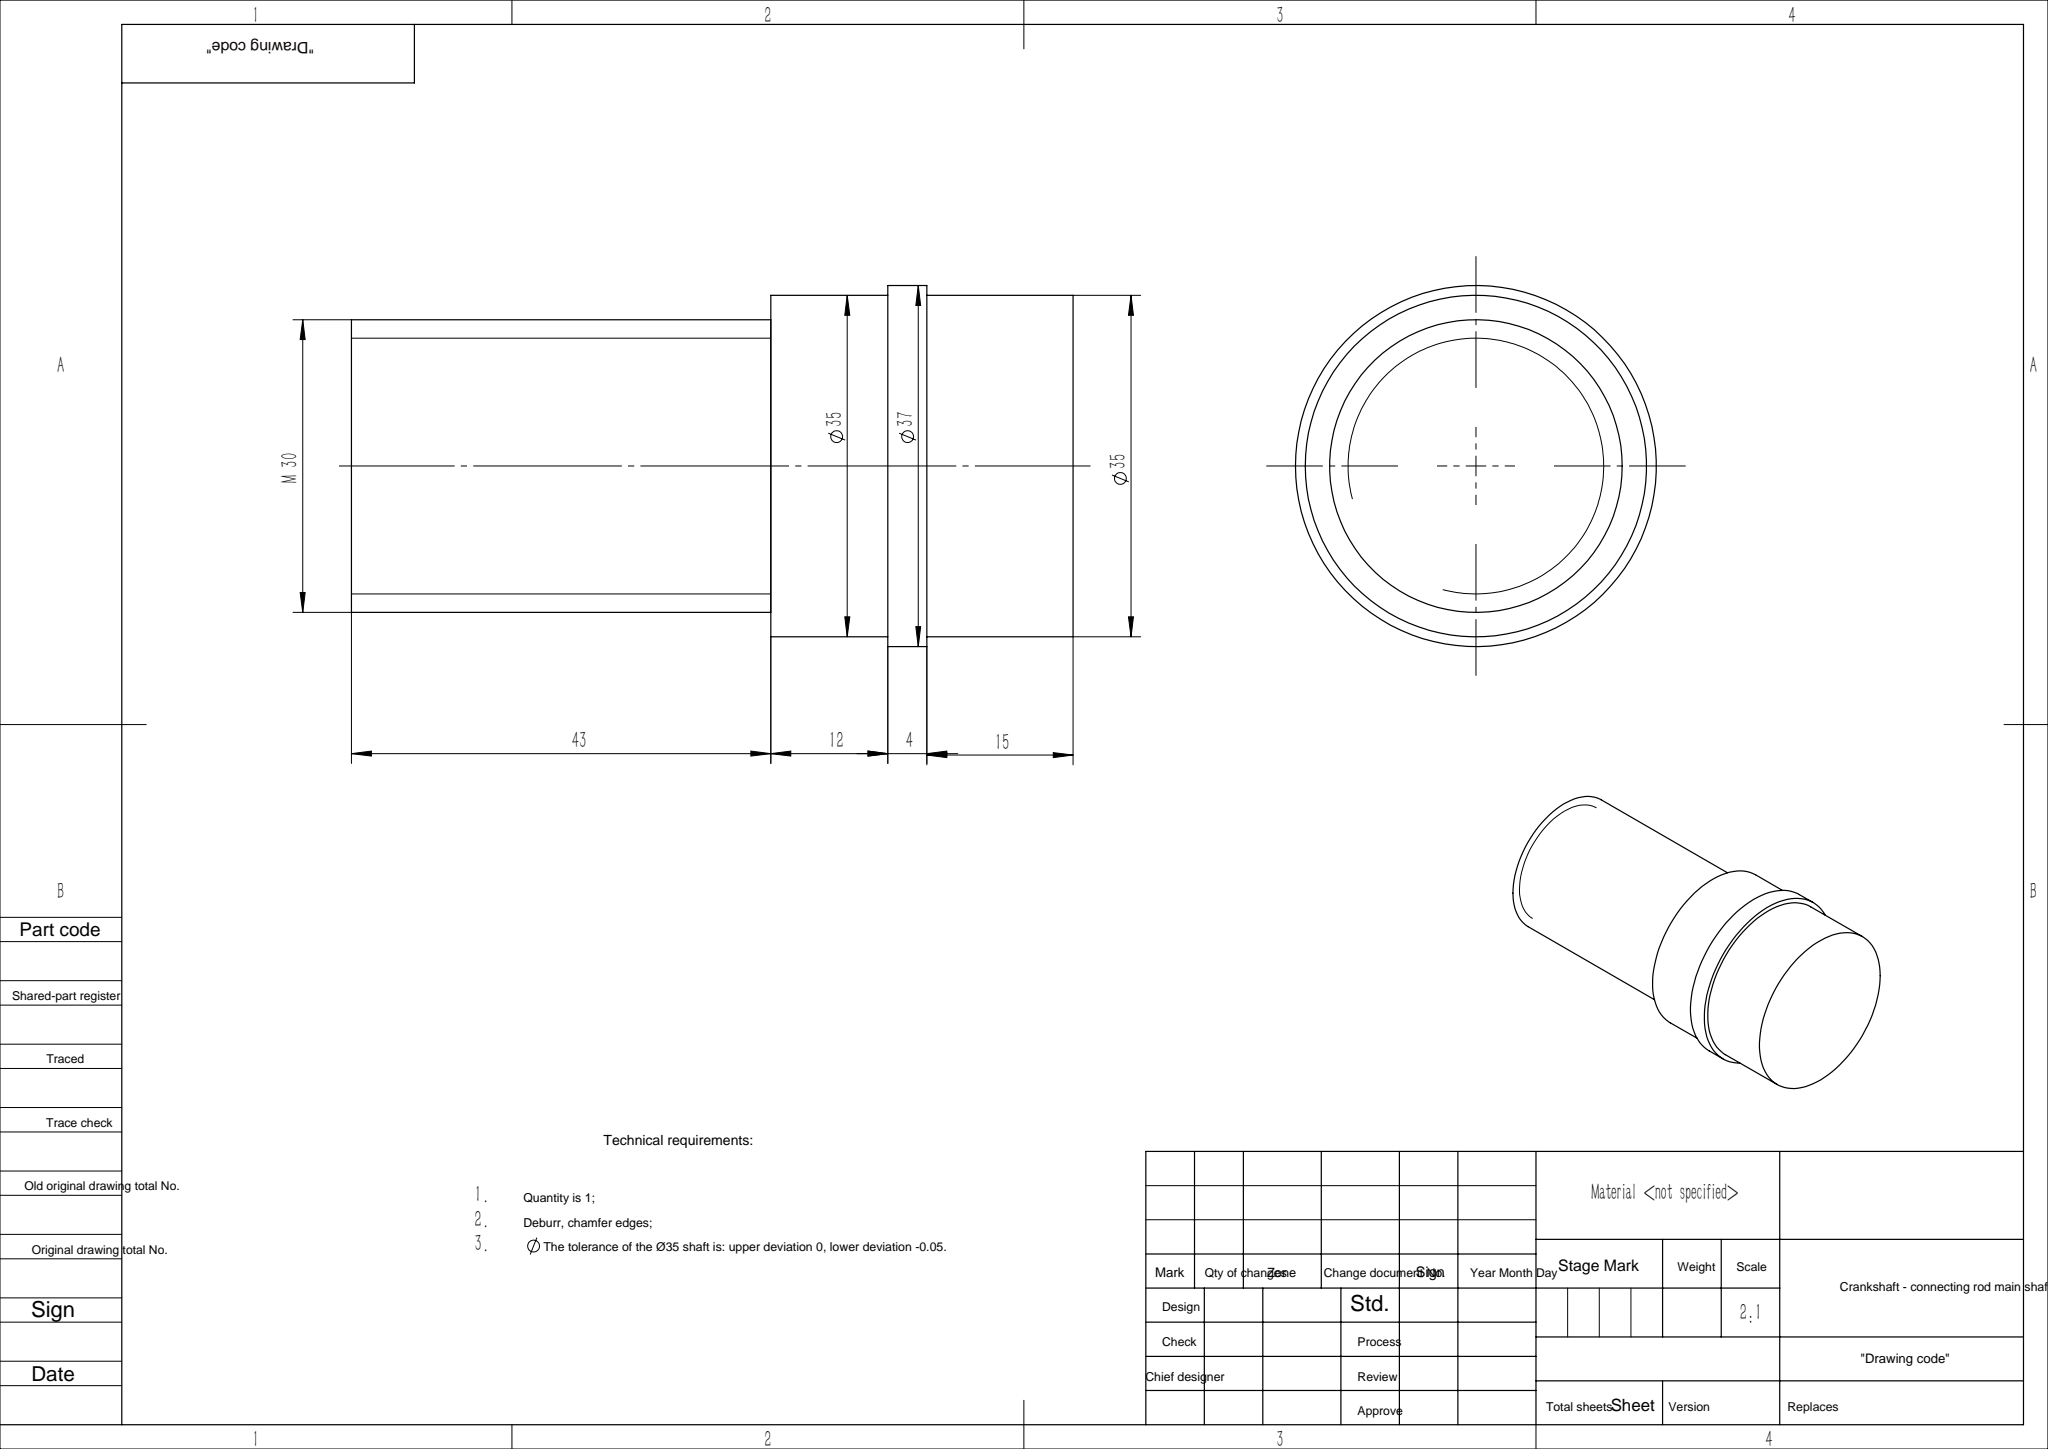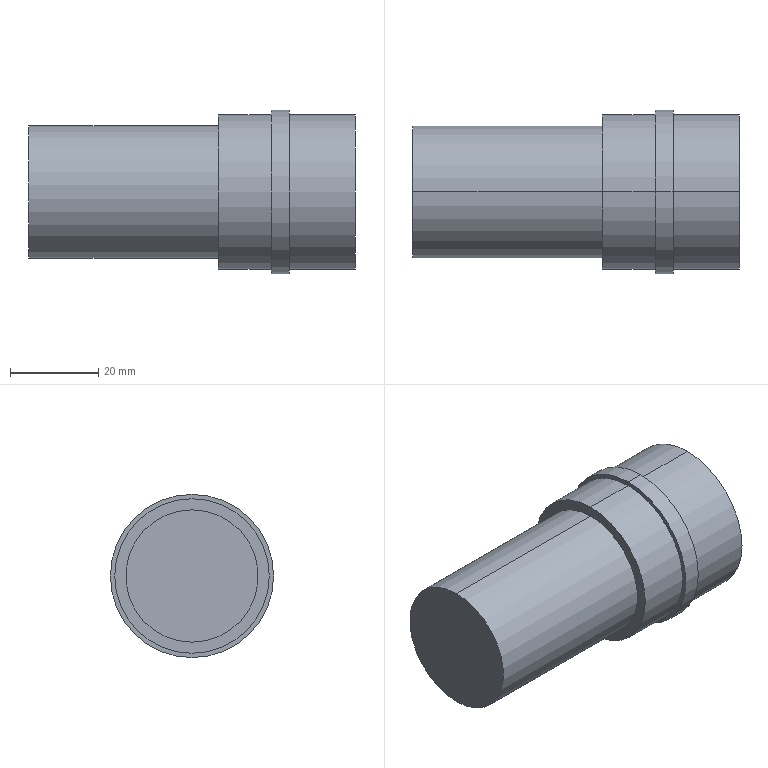Part | SolidWorks | features ICE 2, Extrusion 1 | 1 solid | 13 faces | box 74 x 37 x 37 mm | volume 60673 mm3 | cylinder 8 | plane 5 | commonest cylinder face diameters 35 x4 30 x2 37 x2
STEP:
#1=CARTESIAN_POINT('',(31.,0.,-17.5));
#2=VERTEX_POINT('',#1);
#3=CARTESIAN_POINT('',(31.,0.,17.5));
#4=VERTEX_POINT('',#3);
#5=CARTESIAN_POINT('',(31.,0.,0.));
#6=DIRECTION('',(1.,0.,0.));
#7=DIRECTION('',(0.,0.,-1.));
#8=AXIS2_PLACEMENT_3D('',#5,#6,#7);
#9=CIRCLE('',#8,17.5);
#10=EDGE_CURVE('',#2,#4,#9,.T.);
#11=ORIENTED_EDGE('',*,*,#10,.F.);
#12=CARTESIAN_POINT('',(16.,0.,-17.5));
#13=VERTEX_POINT('',#12);
#14=CARTESIAN_POINT('',(31.,0.,-17.5));
#15=DIRECTION('',(-1.,0.,0.));
#16=VECTOR('',#15,1000.);
#17=LINE('',#14,#16);
#18=EDGE_CURVE('',#2,#13,#17,.T.);
#19=ORIENTED_EDGE('',*,*,#18,.T.);
#20=CARTESIAN_POINT('',(16.,0.,17.5));
#21=VERTEX_POINT('',#20);
#22=CARTESIAN_POINT('',(16.,0.,0.));
#23=DIRECTION('',(1.,0.,0.));
#24=DIRECTION('',(0.,0.,-1.));
#25=AXIS2_PLACEMENT_3D('',#22,#23,#24);
#26=CIRCLE('',#25,17.5);
#27=EDGE_CURVE('',#13,#21,#26,.T.);
#28=ORIENTED_EDGE('',*,*,#27,.T.);
#29=CARTESIAN_POINT('',(31.,0.,17.5));
#30=DIRECTION('',(-1.,0.,0.));
#31=VECTOR('',#30,1000.);
#32=LINE('',#29,#31);
#33=EDGE_CURVE('',#4,#21,#32,.T.);
#34=ORIENTED_EDGE('',*,*,#33,.F.);
#35=EDGE_LOOP('',(#11,#19,#28,#34));
#36=FACE_OUTER_BOUND('',#35,.T.);
#37=CARTESIAN_POINT('',(31.,0.,0.));
#38=DIRECTION('',(-1.,0.,0.));
#39=DIRECTION('',(0.,0.,1.));
#40=AXIS2_PLACEMENT_3D('',#37,#38,#39);
#41=CYLINDRICAL_SURFACE('',#40,17.5);
#42=ADVANCED_FACE('',(#36),#41,.T.);
#43=CARTESIAN_POINT('',(16.,0.,-18.5));
#44=VERTEX_POINT('',#43);
#45=CARTESIAN_POINT('',(16.,0.,18.5));
#46=VERTEX_POINT('',#45);
#47=CARTESIAN_POINT('',(16.,0.,0.));
#48=DIRECTION('',(1.,0.,0.));
#49=DIRECTION('',(0.,0.,-1.));
#50=AXIS2_PLACEMENT_3D('',#47,#48,#49);
#51=CIRCLE('',#50,18.5);
#52=EDGE_CURVE('',#44,#46,#51,.T.);
#53=ORIENTED_EDGE('',*,*,#52,.F.);
#54=CARTESIAN_POINT('',(12.,0.,-18.5));
#55=VERTEX_POINT('',#54);
#56=CARTESIAN_POINT('',(16.,0.,-18.5));
#57=DIRECTION('',(-1.,0.,0.));
#58=VECTOR('',#57,1000.);
#59=LINE('',#56,#58);
#60=EDGE_CURVE('',#44,#55,#59,.T.);
#61=ORIENTED_EDGE('',*,*,#60,.T.);
#62=CARTESIAN_POINT('',(12.,0.,18.5));
#63=VERTEX_POINT('',#62);
#64=CARTESIAN_POINT('',(12.,0.,0.));
#65=DIRECTION('',(1.,0.,0.));
#66=DIRECTION('',(0.,0.,-1.));
#67=AXIS2_PLACEMENT_3D('',#64,#65,#66);
#68=CIRCLE('',#67,18.5);
#69=EDGE_CURVE('',#55,#63,#68,.T.);
#70=ORIENTED_EDGE('',*,*,#69,.T.);
#71=CARTESIAN_POINT('',(16.,0.,18.5));
#72=DIRECTION('',(-1.,0.,0.));
#73=VECTOR('',#72,1000.);
#74=LINE('',#71,#73);
#75=EDGE_CURVE('',#46,#63,#74,.T.);
#76=ORIENTED_EDGE('',*,*,#75,.F.);
#77=EDGE_LOOP('',(#53,#61,#70,#76));
#78=FACE_OUTER_BOUND('',#77,.T.);
#79=CARTESIAN_POINT('',(16.,0.,0.));
#80=DIRECTION('',(-1.,0.,0.));
#81=DIRECTION('',(0.,0.,1.));
#82=AXIS2_PLACEMENT_3D('',#79,#80,#81);
#83=CYLINDRICAL_SURFACE('',#82,18.5);
#84=ADVANCED_FACE('',(#78),#83,.T.);
#85=CARTESIAN_POINT('',(-43.,0.,15.));
#86=VERTEX_POINT('',#85);
#87=CARTESIAN_POINT('',(-43.,0.,-15.));
#88=VERTEX_POINT('',#87);
#89=CARTESIAN_POINT('',(-43.,0.,0.));
#90=DIRECTION('',(-1.,0.,0.));
#91=DIRECTION('',(0.,0.,1.));
#92=AXIS2_PLACEMENT_3D('',#89,#90,#91);
#93=CIRCLE('',#92,15.);
#94=EDGE_CURVE('',#86,#88,#93,.T.);
#95=ORIENTED_EDGE('',*,*,#94,.F.);
#96=CARTESIAN_POINT('',(0.,0.,15.));
#97=VERTEX_POINT('',#96);
#98=CARTESIAN_POINT('',(-43.,0.,15.));
#99=DIRECTION('',(1.,0.,0.));
#100=VECTOR('',#99,1000.);
#101=LINE('',#98,#100);
#102=EDGE_CURVE('',#86,#97,#101,.T.);
#103=ORIENTED_EDGE('',*,*,#102,.T.);
#104=CARTESIAN_POINT('',(0.,0.,-15.));
#105=VERTEX_POINT('',#104);
#106=CARTESIAN_POINT('',(0.,0.,0.));
#107=DIRECTION('',(-1.,0.,0.));
#108=DIRECTION('',(0.,0.,-1.));
#109=AXIS2_PLACEMENT_3D('',#106,#107,#108);
#110=CIRCLE('',#109,15.);
#111=EDGE_CURVE('',#97,#105,#110,.T.);
#112=ORIENTED_EDGE('',*,*,#111,.T.);
#113=CARTESIAN_POINT('',(-43.,0.,-15.));
#114=DIRECTION('',(1.,0.,0.));
#115=VECTOR('',#114,1000.);
#116=LINE('',#113,#115);
#117=EDGE_CURVE('',#88,#105,#116,.T.);
#118=ORIENTED_EDGE('',*,*,#117,.F.);
#119=EDGE_LOOP('',(#95,#103,#112,#118));
#120=FACE_OUTER_BOUND('',#119,.T.);
#121=CARTESIAN_POINT('',(-43.,0.,0.));
#122=DIRECTION('',(1.,0.,0.));
#123=DIRECTION('',(0.,0.,-1.));
#124=AXIS2_PLACEMENT_3D('',#121,#122,#123);
#125=CYLINDRICAL_SURFACE('',#124,15.);
#126=ADVANCED_FACE('',(#120),#125,.T.);
#127=CARTESIAN_POINT('',(12.,0.,-17.5));
#128=VERTEX_POINT('',#127);
#129=CARTESIAN_POINT('',(12.,0.,17.5));
#130=VERTEX_POINT('',#129);
#131=CARTESIAN_POINT('',(12.,0.,0.));
#132=DIRECTION('',(1.,0.,0.));
#133=DIRECTION('',(0.,0.,-1.));
#134=AXIS2_PLACEMENT_3D('',#131,#132,#133);
#135=CIRCLE('',#134,17.5);
#136=EDGE_CURVE('',#128,#130,#135,.T.);
#137=ORIENTED_EDGE('',*,*,#136,.F.);
#138=CARTESIAN_POINT('',(0.,0.,-17.5));
#139=VERTEX_POINT('',#138);
#140=CARTESIAN_POINT('',(31.,0.,-17.5));
#141=DIRECTION('',(-1.,0.,0.));
#142=VECTOR('',#141,1000.);
#143=LINE('',#140,#142);
#144=EDGE_CURVE('',#128,#139,#143,.T.);
#145=ORIENTED_EDGE('',*,*,#144,.T.);
#146=CARTESIAN_POINT('',(0.,0.,17.5));
#147=VERTEX_POINT('',#146);
#148=CARTESIAN_POINT('',(0.,0.,0.));
#149=DIRECTION('',(1.,0.,0.));
#150=DIRECTION('',(0.,0.,-1.));
#151=AXIS2_PLACEMENT_3D('',#148,#149,#150);
#152=CIRCLE('',#151,17.5);
#153=EDGE_CURVE('',#139,#147,#152,.T.);
#154=ORIENTED_EDGE('',*,*,#153,.T.);
#155=CARTESIAN_POINT('',(31.,0.,17.5));
#156=DIRECTION('',(-1.,0.,0.));
#157=VECTOR('',#156,1000.);
#158=LINE('',#155,#157);
#159=EDGE_CURVE('',#130,#147,#158,.T.);
#160=ORIENTED_EDGE('',*,*,#159,.F.);
#161=EDGE_LOOP('',(#137,#145,#154,#160));
#162=FACE_OUTER_BOUND('',#161,.T.);
#163=CARTESIAN_POINT('',(31.,0.,0.));
#164=DIRECTION('',(-1.,0.,0.));
#165=DIRECTION('',(0.,0.,1.));
#166=AXIS2_PLACEMENT_3D('',#163,#164,#165);
#167=CYLINDRICAL_SURFACE('',#166,17.5);
#168=ADVANCED_FACE('',(#162),#167,.T.);
#169=ORIENTED_EDGE('',*,*,#144,.F.);
#170=CARTESIAN_POINT('',(12.,0.,0.));
#171=DIRECTION('',(1.,0.,0.));
#172=DIRECTION('',(0.,0.,-1.));
#173=AXIS2_PLACEMENT_3D('',#170,#171,#172);
#174=CIRCLE('',#173,17.5);
#175=EDGE_CURVE('',#130,#128,#174,.T.);
#176=ORIENTED_EDGE('',*,*,#175,.F.);
#177=ORIENTED_EDGE('',*,*,#159,.T.);
#178=CARTESIAN_POINT('',(0.,0.,0.));
#179=DIRECTION('',(1.,0.,0.));
#180=DIRECTION('',(0.,0.,-1.));
#181=AXIS2_PLACEMENT_3D('',#178,#179,#180);
#182=CIRCLE('',#181,17.5);
#183=EDGE_CURVE('',#147,#139,#182,.T.);
#184=ORIENTED_EDGE('',*,*,#183,.T.);
#185=EDGE_LOOP('',(#169,#176,#177,#184));
#186=FACE_OUTER_BOUND('',#185,.T.);
#187=CARTESIAN_POINT('',(31.,0.,0.));
#188=DIRECTION('',(-1.,0.,0.));
#189=DIRECTION('',(0.,0.,1.));
#190=AXIS2_PLACEMENT_3D('',#187,#188,#189);
#191=CYLINDRICAL_SURFACE('',#190,17.5);
#192=ADVANCED_FACE('',(#186),#191,.T.);
#193=ORIENTED_EDGE('',*,*,#183,.F.);
#194=ORIENTED_EDGE('',*,*,#153,.F.);
#195=EDGE_LOOP('',(#193,#194));
#196=FACE_OUTER_BOUND('',#195,.T.);
#197=CARTESIAN_POINT('',(0.,0.,0.));
#198=DIRECTION('',(-1.,0.,0.));
#199=DIRECTION('',(0.,0.,-1.));
#200=AXIS2_PLACEMENT_3D('',#197,#198,#199);
#201=CIRCLE('',#200,15.);
#202=EDGE_CURVE('',#105,#97,#201,.T.);
#203=ORIENTED_EDGE('',*,*,#202,.F.);
#204=ORIENTED_EDGE('',*,*,#111,.F.);
#205=EDGE_LOOP('',(#203,#204));
#206=FACE_BOUND('',#205,.T.);
#207=CARTESIAN_POINT('',(0.,0.,0.));
#208=DIRECTION('',(1.,0.,0.));
#209=DIRECTION('',(0.,0.,-1.));
#210=AXIS2_PLACEMENT_3D('',#207,#208,#209);
#211=PLANE('',#210);
#212=ADVANCED_FACE('',(#196,#206),#211,.F.);
#213=ORIENTED_EDGE('',*,*,#102,.F.);
#214=CARTESIAN_POINT('',(-43.,0.,0.));
#215=DIRECTION('',(-1.,0.,0.));
#216=DIRECTION('',(0.,0.,1.));
#217=AXIS2_PLACEMENT_3D('',#214,#215,#216);
#218=CIRCLE('',#217,15.);
#219=EDGE_CURVE('',#88,#86,#218,.T.);
#220=ORIENTED_EDGE('',*,*,#219,.F.);
#221=ORIENTED_EDGE('',*,*,#117,.T.);
#222=ORIENTED_EDGE('',*,*,#202,.T.);
#223=EDGE_LOOP('',(#213,#220,#221,#222));
#224=FACE_OUTER_BOUND('',#223,.T.);
#225=CARTESIAN_POINT('',(-43.,0.,0.));
#226=DIRECTION('',(1.,0.,0.));
#227=DIRECTION('',(0.,0.,-1.));
#228=AXIS2_PLACEMENT_3D('',#225,#226,#227);
#229=CYLINDRICAL_SURFACE('',#228,15.);
#230=ADVANCED_FACE('',(#224),#229,.T.);
#231=ORIENTED_EDGE('',*,*,#219,.T.);
#232=ORIENTED_EDGE('',*,*,#94,.T.);
#233=EDGE_LOOP('',(#231,#232));
#234=FACE_OUTER_BOUND('',#233,.T.);
#235=CARTESIAN_POINT('',(-43.,0.,0.));
#236=DIRECTION('',(-1.,0.,0.));
#237=DIRECTION('',(0.,0.,1.));
#238=AXIS2_PLACEMENT_3D('',#235,#236,#237);
#239=PLANE('',#238);
#240=ADVANCED_FACE('',(#234),#239,.T.);
#241=CARTESIAN_POINT('',(16.,0.,0.));
#242=DIRECTION('',(1.,0.,0.));
#243=DIRECTION('',(0.,0.,-1.));
#244=AXIS2_PLACEMENT_3D('',#241,#242,#243);
#245=CIRCLE('',#244,18.5);
#246=EDGE_CURVE('',#46,#44,#245,.T.);
#247=ORIENTED_EDGE('',*,*,#246,.T.);
#248=ORIENTED_EDGE('',*,*,#52,.T.);
#249=EDGE_LOOP('',(#247,#248));
#250=FACE_OUTER_BOUND('',#249,.T.);
#251=CARTESIAN_POINT('',(16.,0.,0.));
#252=DIRECTION('',(1.,0.,0.));
#253=DIRECTION('',(0.,0.,-1.));
#254=AXIS2_PLACEMENT_3D('',#251,#252,#253);
#255=CIRCLE('',#254,17.5);
#256=EDGE_CURVE('',#21,#13,#255,.T.);
#257=ORIENTED_EDGE('',*,*,#256,.F.);
#258=ORIENTED_EDGE('',*,*,#27,.F.);
#259=EDGE_LOOP('',(#257,#258));
#260=FACE_BOUND('',#259,.T.);
#261=CARTESIAN_POINT('',(16.,0.,0.));
#262=DIRECTION('',(1.,0.,0.));
#263=DIRECTION('',(0.,0.,-1.));
#264=AXIS2_PLACEMENT_3D('',#261,#262,#263);
#265=PLANE('',#264);
#266=ADVANCED_FACE('',(#250,#260),#265,.T.);
#267=CARTESIAN_POINT('',(12.,0.,0.));
#268=DIRECTION('',(1.,0.,0.));
#269=DIRECTION('',(0.,0.,-1.));
#270=AXIS2_PLACEMENT_3D('',#267,#268,#269);
#271=CIRCLE('',#270,18.5);
#272=EDGE_CURVE('',#63,#55,#271,.T.);
#273=ORIENTED_EDGE('',*,*,#272,.F.);
#274=ORIENTED_EDGE('',*,*,#69,.F.);
#275=EDGE_LOOP('',(#273,#274));
#276=FACE_OUTER_BOUND('',#275,.T.);
#277=ORIENTED_EDGE('',*,*,#175,.T.);
#278=ORIENTED_EDGE('',*,*,#136,.T.);
#279=EDGE_LOOP('',(#277,#278));
#280=FACE_BOUND('',#279,.T.);
#281=CARTESIAN_POINT('',(12.,0.,0.));
#282=DIRECTION('',(1.,0.,0.));
#283=DIRECTION('',(0.,0.,-1.));
#284=AXIS2_PLACEMENT_3D('',#281,#282,#283);
#285=PLANE('',#284);
#286=ADVANCED_FACE('',(#276,#280),#285,.F.);
#287=ORIENTED_EDGE('',*,*,#60,.F.);
#288=ORIENTED_EDGE('',*,*,#246,.F.);
#289=ORIENTED_EDGE('',*,*,#75,.T.);
#290=ORIENTED_EDGE('',*,*,#272,.T.);
#291=EDGE_LOOP('',(#287,#288,#289,#290));
#292=FACE_OUTER_BOUND('',#291,.T.);
#293=CARTESIAN_POINT('',(16.,0.,0.));
#294=DIRECTION('',(-1.,0.,0.));
#295=DIRECTION('',(0.,0.,1.));
#296=AXIS2_PLACEMENT_3D('',#293,#294,#295);
#297=CYLINDRICAL_SURFACE('',#296,18.5);
#298=ADVANCED_FACE('',(#292),#297,.T.);
#299=CARTESIAN_POINT('',(31.,0.,0.));
#300=DIRECTION('',(1.,0.,0.));
#301=DIRECTION('',(0.,0.,-1.));
#302=AXIS2_PLACEMENT_3D('',#299,#300,#301);
#303=CIRCLE('',#302,17.5);
#304=EDGE_CURVE('',#4,#2,#303,.T.);
#305=ORIENTED_EDGE('',*,*,#304,.T.);
#306=ORIENTED_EDGE('',*,*,#10,.T.);
#307=EDGE_LOOP('',(#305,#306));
#308=FACE_OUTER_BOUND('',#307,.T.);
#309=CARTESIAN_POINT('',(31.,0.,0.));
#310=DIRECTION('',(1.,0.,0.));
#311=DIRECTION('',(0.,0.,-1.));
#312=AXIS2_PLACEMENT_3D('',#309,#310,#311);
#313=PLANE('',#312);
#314=ADVANCED_FACE('',(#308),#313,.T.);
#315=ORIENTED_EDGE('',*,*,#18,.F.);
#316=ORIENTED_EDGE('',*,*,#304,.F.);
#317=ORIENTED_EDGE('',*,*,#33,.T.);
#318=ORIENTED_EDGE('',*,*,#256,.T.);
#319=EDGE_LOOP('',(#315,#316,#317,#318));
#320=FACE_OUTER_BOUND('',#319,.T.);
#321=CARTESIAN_POINT('',(31.,0.,0.));
#322=DIRECTION('',(-1.,0.,0.));
#323=DIRECTION('',(0.,0.,1.));
#324=AXIS2_PLACEMENT_3D('',#321,#322,#323);
#325=CYLINDRICAL_SURFACE('',#324,17.5);
#326=ADVANCED_FACE('',(#320),#325,.T.);
#327=CLOSED_SHELL('',(#42,#84,#126,#168,#192,#212,#230,#240,#266,#286,#298,#314,#326));
#328=MANIFOLD_SOLID_BREP('',#327);
#329=CARTESIAN_POINT('',(0.,0.,0.));
#330=DIRECTION('',(0.,0.,1.));
#331=DIRECTION('',(1.,0.,0.));
#332=AXIS2_PLACEMENT_3D('',#329,#330,#331);
#333=(LENGTH_UNIT()NAMED_UNIT(*)SI_UNIT(.MILLI.,.METRE.));
#334=UNCERTAINTY_MEASURE_WITH_UNIT(LENGTH_MEASURE(0.00001),#333,'','');
#335=(NAMED_UNIT(*)PLANE_ANGLE_UNIT()SI_UNIT($,.RADIAN.));
#336=(NAMED_UNIT(*)SI_UNIT($,.STERADIAN.)SOLID_ANGLE_UNIT());
#337=(GEOMETRIC_REPRESENTATION_CONTEXT(3)GLOBAL_UNCERTAINTY_ASSIGNED_CONTEXT((#334))GLOBAL_UNIT_ASSIGNED_CONTEXT((#333,#335,#336))REPRESENTATION_CONTEXT('',''));
#338=ADVANCED_BREP_SHAPE_REPRESENTATION('',(#328,#332),#337);